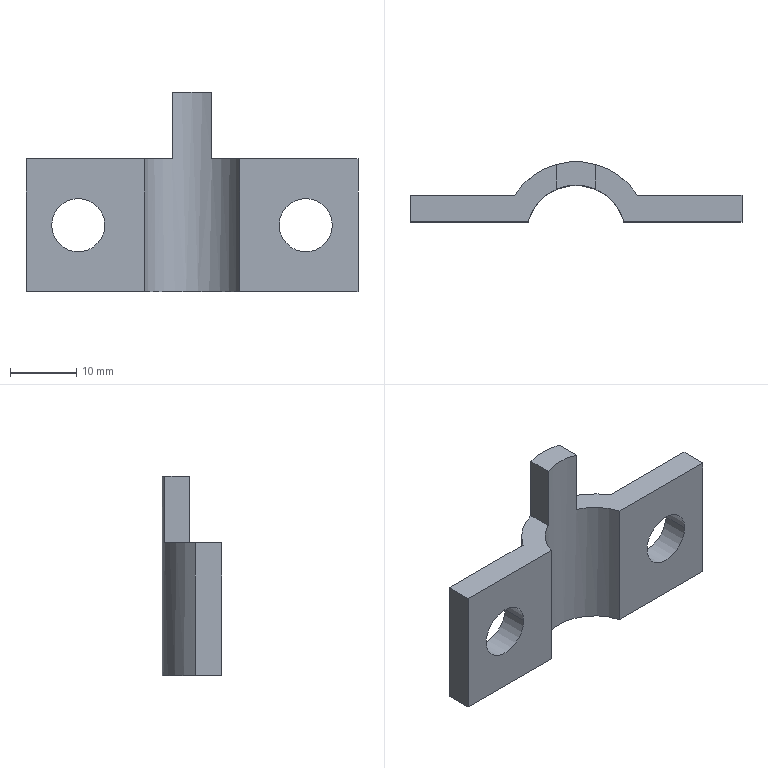Part | SolidWorks | features ICE 2, Extrusion 1 | 1 solid | 18 faces | box 50 x 9.031 x 30 mm | volume 3952 mm3 | plane 12 | cylinder 6 | commonest cylinder face diameters 8 x4 15 x1 22.063 x1
STEP:
#1=CARTESIAN_POINT('',(21.128,4.,10.));
#2=VERTEX_POINT('',#1);
#3=CARTESIAN_POINT('',(13.128,4.,10.));
#4=VERTEX_POINT('',#3);
#5=CARTESIAN_POINT('',(17.128,4.,10.));
#6=DIRECTION('',(0.,1.,0.));
#7=DIRECTION('',(-1.,0.,0.));
#8=AXIS2_PLACEMENT_3D('',#5,#6,#7);
#9=CIRCLE('',#8,4.);
#10=EDGE_CURVE('',#2,#4,#9,.T.);
#11=ORIENTED_EDGE('',*,*,#10,.F.);
#12=CARTESIAN_POINT('',(21.128,8.,10.));
#13=VERTEX_POINT('',#12);
#14=CARTESIAN_POINT('',(21.128,4.,10.));
#15=DIRECTION('',(0.,1.,0.));
#16=VECTOR('',#15,1000.);
#17=LINE('',#14,#16);
#18=EDGE_CURVE('',#2,#13,#17,.T.);
#19=ORIENTED_EDGE('',*,*,#18,.T.);
#20=CARTESIAN_POINT('',(13.128,8.,10.));
#21=VERTEX_POINT('',#20);
#22=CARTESIAN_POINT('',(17.128,8.,10.));
#23=DIRECTION('',(0.,1.,0.));
#24=DIRECTION('',(-1.,0.,0.));
#25=AXIS2_PLACEMENT_3D('',#22,#23,#24);
#26=CIRCLE('',#25,4.);
#27=EDGE_CURVE('',#13,#21,#26,.T.);
#28=ORIENTED_EDGE('',*,*,#27,.T.);
#29=CARTESIAN_POINT('',(13.128,4.,10.));
#30=DIRECTION('',(0.,1.,0.));
#31=VECTOR('',#30,1000.);
#32=LINE('',#29,#31);
#33=EDGE_CURVE('',#4,#21,#32,.T.);
#34=ORIENTED_EDGE('',*,*,#33,.F.);
#35=EDGE_LOOP('',(#11,#19,#28,#34));
#36=FACE_OUTER_BOUND('',#35,.T.);
#37=CARTESIAN_POINT('',(17.128,4.,10.));
#38=DIRECTION('',(0.,1.,0.));
#39=DIRECTION('',(-1.,0.,0.));
#40=AXIS2_PLACEMENT_3D('',#37,#38,#39);
#41=CYLINDRICAL_SURFACE('',#40,4.);
#42=ADVANCED_FACE('',(#36),#41,.F.);
#43=CARTESIAN_POINT('',(-13.128,4.,10.));
#44=VERTEX_POINT('',#43);
#45=CARTESIAN_POINT('',(-21.128,4.,10.));
#46=VERTEX_POINT('',#45);
#47=CARTESIAN_POINT('',(-17.128,4.,10.));
#48=DIRECTION('',(0.,1.,0.));
#49=DIRECTION('',(-1.,0.,0.));
#50=AXIS2_PLACEMENT_3D('',#47,#48,#49);
#51=CIRCLE('',#50,4.);
#52=EDGE_CURVE('',#44,#46,#51,.T.);
#53=ORIENTED_EDGE('',*,*,#52,.F.);
#54=CARTESIAN_POINT('',(-13.128,8.,10.));
#55=VERTEX_POINT('',#54);
#56=CARTESIAN_POINT('',(-13.128,4.,10.));
#57=DIRECTION('',(0.,1.,0.));
#58=VECTOR('',#57,1000.);
#59=LINE('',#56,#58);
#60=EDGE_CURVE('',#44,#55,#59,.T.);
#61=ORIENTED_EDGE('',*,*,#60,.T.);
#62=CARTESIAN_POINT('',(-21.128,8.,10.));
#63=VERTEX_POINT('',#62);
#64=CARTESIAN_POINT('',(-17.128,8.,10.));
#65=DIRECTION('',(0.,1.,0.));
#66=DIRECTION('',(-1.,0.,0.));
#67=AXIS2_PLACEMENT_3D('',#64,#65,#66);
#68=CIRCLE('',#67,4.);
#69=EDGE_CURVE('',#55,#63,#68,.T.);
#70=ORIENTED_EDGE('',*,*,#69,.T.);
#71=CARTESIAN_POINT('',(-21.128,4.,10.));
#72=DIRECTION('',(0.,1.,0.));
#73=VECTOR('',#72,1000.);
#74=LINE('',#71,#73);
#75=EDGE_CURVE('',#46,#63,#74,.T.);
#76=ORIENTED_EDGE('',*,*,#75,.F.);
#77=EDGE_LOOP('',(#53,#61,#70,#76));
#78=FACE_OUTER_BOUND('',#77,.T.);
#79=CARTESIAN_POINT('',(-17.128,4.,10.));
#80=DIRECTION('',(0.,1.,0.));
#81=DIRECTION('',(-1.,0.,0.));
#82=AXIS2_PLACEMENT_3D('',#79,#80,#81);
#83=CYLINDRICAL_SURFACE('',#82,4.);
#84=ADVANCED_FACE('',(#78),#83,.F.);
#85=CARTESIAN_POINT('',(7.228,4.,20.));
#86=VERTEX_POINT('',#85);
#87=CARTESIAN_POINT('',(7.228,4.,0.));
#88=VERTEX_POINT('',#87);
#89=CARTESIAN_POINT('',(7.228,4.,30.));
#90=DIRECTION('',(0.,0.,-1.));
#91=VECTOR('',#90,1000.);
#92=LINE('',#89,#91);
#93=EDGE_CURVE('',#86,#88,#92,.T.);
#94=ORIENTED_EDGE('',*,*,#93,.F.);
#95=CARTESIAN_POINT('',(3.,8.874,20.));
#96=VERTEX_POINT('',#95);
#97=CARTESIAN_POINT('',(0.,2.,20.));
#98=DIRECTION('',(0.,0.,1.));
#99=DIRECTION('',(-1.,0.,0.));
#100=AXIS2_PLACEMENT_3D('',#97,#98,#99);
#101=CIRCLE('',#100,7.5);
#102=EDGE_CURVE('',#86,#96,#101,.T.);
#103=ORIENTED_EDGE('',*,*,#102,.T.);
#104=CARTESIAN_POINT('',(3.,8.874,30.));
#105=VERTEX_POINT('',#104);
#106=CARTESIAN_POINT('',(3.,8.874,30.));
#107=DIRECTION('',(0.,0.,1.));
#108=VECTOR('',#107,1000.);
#109=LINE('',#106,#108);
#110=EDGE_CURVE('',#96,#105,#109,.T.);
#111=ORIENTED_EDGE('',*,*,#110,.T.);
#112=CARTESIAN_POINT('',(-3.,8.874,30.));
#113=VERTEX_POINT('',#112);
#114=CARTESIAN_POINT('',(0.,2.,30.));
#115=DIRECTION('',(0.,0.,-1.));
#116=DIRECTION('',(1.,0.,0.));
#117=AXIS2_PLACEMENT_3D('',#114,#115,#116);
#118=CIRCLE('',#117,7.5);
#119=EDGE_CURVE('',#113,#105,#118,.T.);
#120=ORIENTED_EDGE('',*,*,#119,.F.);
#121=CARTESIAN_POINT('',(-3.,8.874,20.));
#122=VERTEX_POINT('',#121);
#123=CARTESIAN_POINT('',(-3.,8.874,30.));
#124=DIRECTION('',(0.,0.,-1.));
#125=VECTOR('',#124,1000.);
#126=LINE('',#123,#125);
#127=EDGE_CURVE('',#113,#122,#126,.T.);
#128=ORIENTED_EDGE('',*,*,#127,.T.);
#129=CARTESIAN_POINT('',(-7.228,4.,20.));
#130=VERTEX_POINT('',#129);
#131=CARTESIAN_POINT('',(0.,2.,20.));
#132=DIRECTION('',(0.,0.,1.));
#133=DIRECTION('',(-1.,0.,0.));
#134=AXIS2_PLACEMENT_3D('',#131,#132,#133);
#135=CIRCLE('',#134,7.5);
#136=EDGE_CURVE('',#122,#130,#135,.T.);
#137=ORIENTED_EDGE('',*,*,#136,.T.);
#138=CARTESIAN_POINT('',(-7.228,4.,0.));
#139=VERTEX_POINT('',#138);
#140=CARTESIAN_POINT('',(-7.228,4.,30.));
#141=DIRECTION('',(0.,0.,-1.));
#142=VECTOR('',#141,1000.);
#143=LINE('',#140,#142);
#144=EDGE_CURVE('',#130,#139,#143,.T.);
#145=ORIENTED_EDGE('',*,*,#144,.T.);
#146=CARTESIAN_POINT('',(0.,2.,0.));
#147=DIRECTION('',(0.,0.,-1.));
#148=DIRECTION('',(1.,0.,0.));
#149=AXIS2_PLACEMENT_3D('',#146,#147,#148);
#150=CIRCLE('',#149,7.5);
#151=EDGE_CURVE('',#139,#88,#150,.T.);
#152=ORIENTED_EDGE('',*,*,#151,.T.);
#153=EDGE_LOOP('',(#94,#103,#111,#120,#128,#137,#145,#152));
#154=FACE_OUTER_BOUND('',#153,.T.);
#155=CARTESIAN_POINT('',(0.,2.,30.));
#156=DIRECTION('',(0.,0.,-1.));
#157=DIRECTION('',(-1.,0.,0.));
#158=AXIS2_PLACEMENT_3D('',#155,#156,#157);
#159=CYLINDRICAL_SURFACE('',#158,7.5);
#160=ADVANCED_FACE('',(#154),#159,.F.);
#161=CARTESIAN_POINT('',(17.128,4.,10.));
#162=DIRECTION('',(0.,1.,0.));
#163=DIRECTION('',(-1.,0.,0.));
#164=AXIS2_PLACEMENT_3D('',#161,#162,#163);
#165=CIRCLE('',#164,4.);
#166=EDGE_CURVE('',#4,#2,#165,.T.);
#167=ORIENTED_EDGE('',*,*,#166,.T.);
#168=ORIENTED_EDGE('',*,*,#10,.T.);
#169=EDGE_LOOP('',(#167,#168));
#170=FACE_BOUND('',#169,.T.);
#171=CARTESIAN_POINT('',(25.,4.,20.));
#172=VERTEX_POINT('',#171);
#173=CARTESIAN_POINT('',(25.,4.,0.));
#174=VERTEX_POINT('',#173);
#175=CARTESIAN_POINT('',(25.,4.,30.));
#176=DIRECTION('',(0.,0.,-1.));
#177=VECTOR('',#176,1000.);
#178=LINE('',#175,#177);
#179=EDGE_CURVE('',#172,#174,#178,.T.);
#180=ORIENTED_EDGE('',*,*,#179,.F.);
#181=CARTESIAN_POINT('',(3.,4.,20.));
#182=DIRECTION('',(1.,0.,0.));
#183=VECTOR('',#182,1000.);
#184=LINE('',#181,#183);
#185=EDGE_CURVE('',#86,#172,#184,.T.);
#186=ORIENTED_EDGE('',*,*,#185,.F.);
#187=ORIENTED_EDGE('',*,*,#93,.T.);
#188=CARTESIAN_POINT('',(7.228,4.,0.));
#189=DIRECTION('',(1.,0.,0.));
#190=VECTOR('',#189,1000.);
#191=LINE('',#188,#190);
#192=EDGE_CURVE('',#88,#174,#191,.T.);
#193=ORIENTED_EDGE('',*,*,#192,.T.);
#194=EDGE_LOOP('',(#180,#186,#187,#193));
#195=FACE_OUTER_BOUND('',#194,.T.);
#196=CARTESIAN_POINT('',(7.228,4.,30.));
#197=DIRECTION('',(0.,1.,0.));
#198=DIRECTION('',(0.,0.,1.));
#199=AXIS2_PLACEMENT_3D('',#196,#197,#198);
#200=PLANE('',#199);
#201=ADVANCED_FACE('',(#170,#195),#200,.F.);
#202=CARTESIAN_POINT('',(25.,8.,20.));
#203=VERTEX_POINT('',#202);
#204=CARTESIAN_POINT('',(25.,8.,0.));
#205=VERTEX_POINT('',#204);
#206=CARTESIAN_POINT('',(25.,8.,30.));
#207=DIRECTION('',(0.,0.,-1.));
#208=VECTOR('',#207,1000.);
#209=LINE('',#206,#208);
#210=EDGE_CURVE('',#203,#205,#209,.T.);
#211=ORIENTED_EDGE('',*,*,#210,.F.);
#212=CARTESIAN_POINT('',(25.,13.031,20.));
#213=DIRECTION('',(0.,-1.,0.));
#214=VECTOR('',#213,1000.);
#215=LINE('',#212,#214);
#216=EDGE_CURVE('',#203,#172,#215,.T.);
#217=ORIENTED_EDGE('',*,*,#216,.T.);
#218=ORIENTED_EDGE('',*,*,#179,.T.);
#219=CARTESIAN_POINT('',(25.,8.,0.));
#220=DIRECTION('',(0.,1.,0.));
#221=VECTOR('',#220,1000.);
#222=LINE('',#219,#221);
#223=EDGE_CURVE('',#174,#205,#222,.T.);
#224=ORIENTED_EDGE('',*,*,#223,.T.);
#225=EDGE_LOOP('',(#211,#217,#218,#224));
#226=FACE_OUTER_BOUND('',#225,.T.);
#227=CARTESIAN_POINT('',(25.,8.,30.));
#228=DIRECTION('',(-1.,0.,0.));
#229=DIRECTION('',(0.,0.,1.));
#230=AXIS2_PLACEMENT_3D('',#227,#228,#229);
#231=PLANE('',#230);
#232=ADVANCED_FACE('',(#226),#231,.F.);
#233=CARTESIAN_POINT('',(17.128,8.,10.));
#234=DIRECTION('',(0.,1.,0.));
#235=DIRECTION('',(-1.,0.,0.));
#236=AXIS2_PLACEMENT_3D('',#233,#234,#235);
#237=CIRCLE('',#236,4.);
#238=EDGE_CURVE('',#21,#13,#237,.T.);
#239=ORIENTED_EDGE('',*,*,#238,.F.);
#240=ORIENTED_EDGE('',*,*,#27,.F.);
#241=EDGE_LOOP('',(#239,#240));
#242=FACE_BOUND('',#241,.T.);
#243=CARTESIAN_POINT('',(9.257,8.,20.));
#244=VERTEX_POINT('',#243);
#245=CARTESIAN_POINT('',(9.257,8.,0.));
#246=VERTEX_POINT('',#245);
#247=CARTESIAN_POINT('',(9.257,8.,30.));
#248=DIRECTION('',(0.,0.,-1.));
#249=VECTOR('',#248,1000.);
#250=LINE('',#247,#249);
#251=EDGE_CURVE('',#244,#246,#250,.T.);
#252=ORIENTED_EDGE('',*,*,#251,.F.);
#253=CARTESIAN_POINT('',(25.,8.,20.));
#254=DIRECTION('',(1.,0.,0.));
#255=VECTOR('',#254,1000.);
#256=LINE('',#253,#255);
#257=EDGE_CURVE('',#244,#203,#256,.T.);
#258=ORIENTED_EDGE('',*,*,#257,.T.);
#259=ORIENTED_EDGE('',*,*,#210,.T.);
#260=CARTESIAN_POINT('',(25.,8.,0.));
#261=DIRECTION('',(-1.,0.,0.));
#262=VECTOR('',#261,1000.);
#263=LINE('',#260,#262);
#264=EDGE_CURVE('',#205,#246,#263,.T.);
#265=ORIENTED_EDGE('',*,*,#264,.T.);
#266=EDGE_LOOP('',(#252,#258,#259,#265));
#267=FACE_OUTER_BOUND('',#266,.T.);
#268=CARTESIAN_POINT('',(25.,8.,30.));
#269=DIRECTION('',(0.,-1.,0.));
#270=DIRECTION('',(1.,0.,0.));
#271=AXIS2_PLACEMENT_3D('',#268,#269,#270);
#272=PLANE('',#271);
#273=ADVANCED_FACE('',(#242,#267),#272,.F.);
#274=CARTESIAN_POINT('',(3.,12.616,30.));
#275=VERTEX_POINT('',#274);
#276=CARTESIAN_POINT('',(3.,12.616,20.));
#277=VERTEX_POINT('',#276);
#278=CARTESIAN_POINT('',(3.,12.616,30.));
#279=DIRECTION('',(0.,0.,-1.));
#280=VECTOR('',#279,1000.);
#281=LINE('',#278,#280);
#282=EDGE_CURVE('',#275,#277,#281,.T.);
#283=ORIENTED_EDGE('',*,*,#282,.T.);
#284=CARTESIAN_POINT('',(0.,2.,20.));
#285=DIRECTION('',(0.,0.,-1.));
#286=DIRECTION('',(-1.,0.,0.));
#287=AXIS2_PLACEMENT_3D('',#284,#285,#286);
#288=CIRCLE('',#287,11.031);
#289=EDGE_CURVE('',#277,#244,#288,.T.);
#290=ORIENTED_EDGE('',*,*,#289,.T.);
#291=ORIENTED_EDGE('',*,*,#251,.T.);
#292=CARTESIAN_POINT('',(-9.257,8.,0.));
#293=VERTEX_POINT('',#292);
#294=CARTESIAN_POINT('',(0.,2.,0.));
#295=DIRECTION('',(0.,0.,1.));
#296=DIRECTION('',(1.,0.,0.));
#297=AXIS2_PLACEMENT_3D('',#294,#295,#296);
#298=CIRCLE('',#297,11.031);
#299=EDGE_CURVE('',#246,#293,#298,.T.);
#300=ORIENTED_EDGE('',*,*,#299,.T.);
#301=CARTESIAN_POINT('',(-9.257,8.,20.));
#302=VERTEX_POINT('',#301);
#303=CARTESIAN_POINT('',(-9.257,8.,30.));
#304=DIRECTION('',(0.,0.,-1.));
#305=VECTOR('',#304,1000.);
#306=LINE('',#303,#305);
#307=EDGE_CURVE('',#302,#293,#306,.T.);
#308=ORIENTED_EDGE('',*,*,#307,.F.);
#309=CARTESIAN_POINT('',(-3.,12.616,20.));
#310=VERTEX_POINT('',#309);
#311=CARTESIAN_POINT('',(0.,2.,20.));
#312=DIRECTION('',(0.,0.,-1.));
#313=DIRECTION('',(-1.,0.,0.));
#314=AXIS2_PLACEMENT_3D('',#311,#312,#313);
#315=CIRCLE('',#314,11.031);
#316=EDGE_CURVE('',#302,#310,#315,.T.);
#317=ORIENTED_EDGE('',*,*,#316,.T.);
#318=CARTESIAN_POINT('',(-3.,12.616,30.));
#319=VERTEX_POINT('',#318);
#320=CARTESIAN_POINT('',(-3.,12.616,30.));
#321=DIRECTION('',(0.,0.,1.));
#322=VECTOR('',#321,1000.);
#323=LINE('',#320,#322);
#324=EDGE_CURVE('',#310,#319,#323,.T.);
#325=ORIENTED_EDGE('',*,*,#324,.T.);
#326=CARTESIAN_POINT('',(0.,2.,30.));
#327=DIRECTION('',(0.,0.,1.));
#328=DIRECTION('',(1.,0.,0.));
#329=AXIS2_PLACEMENT_3D('',#326,#327,#328);
#330=CIRCLE('',#329,11.031);
#331=EDGE_CURVE('',#275,#319,#330,.T.);
#332=ORIENTED_EDGE('',*,*,#331,.F.);
#333=EDGE_LOOP('',(#283,#290,#291,#300,#308,#317,#325,#332));
#334=FACE_OUTER_BOUND('',#333,.T.);
#335=CARTESIAN_POINT('',(0.,2.,30.));
#336=DIRECTION('',(0.,0.,-1.));
#337=DIRECTION('',(-1.,0.,0.));
#338=AXIS2_PLACEMENT_3D('',#335,#336,#337);
#339=CYLINDRICAL_SURFACE('',#338,11.031);
#340=ADVANCED_FACE('',(#334),#339,.T.);
#341=CARTESIAN_POINT('',(-17.128,8.,10.));
#342=DIRECTION('',(0.,1.,0.));
#343=DIRECTION('',(-1.,0.,0.));
#344=AXIS2_PLACEMENT_3D('',#341,#342,#343);
#345=CIRCLE('',#344,4.);
#346=EDGE_CURVE('',#63,#55,#345,.T.);
#347=ORIENTED_EDGE('',*,*,#346,.F.);
#348=ORIENTED_EDGE('',*,*,#69,.F.);
#349=EDGE_LOOP('',(#347,#348));
#350=FACE_BOUND('',#349,.T.);
#351=CARTESIAN_POINT('',(-25.,8.,20.));
#352=VERTEX_POINT('',#351);
#353=CARTESIAN_POINT('',(-25.,8.,0.));
#354=VERTEX_POINT('',#353);
#355=CARTESIAN_POINT('',(-25.,8.,30.));
#356=DIRECTION('',(0.,0.,-1.));
#357=VECTOR('',#356,1000.);
#358=LINE('',#355,#357);
#359=EDGE_CURVE('',#352,#354,#358,.T.);
#360=ORIENTED_EDGE('',*,*,#359,.F.);
#361=CARTESIAN_POINT('',(-25.,8.,20.));
#362=DIRECTION('',(1.,0.,0.));
#363=VECTOR('',#362,1000.);
#364=LINE('',#361,#363);
#365=EDGE_CURVE('',#352,#302,#364,.T.);
#366=ORIENTED_EDGE('',*,*,#365,.T.);
#367=ORIENTED_EDGE('',*,*,#307,.T.);
#368=CARTESIAN_POINT('',(-25.,8.,0.));
#369=DIRECTION('',(-1.,0.,0.));
#370=VECTOR('',#369,1000.);
#371=LINE('',#368,#370);
#372=EDGE_CURVE('',#293,#354,#371,.T.);
#373=ORIENTED_EDGE('',*,*,#372,.T.);
#374=EDGE_LOOP('',(#360,#366,#367,#373));
#375=FACE_OUTER_BOUND('',#374,.T.);
#376=CARTESIAN_POINT('',(-25.,8.,30.));
#377=DIRECTION('',(0.,-1.,0.));
#378=DIRECTION('',(0.,0.,-1.));
#379=AXIS2_PLACEMENT_3D('',#376,#377,#378);
#380=PLANE('',#379);
#381=ADVANCED_FACE('',(#350,#375),#380,.F.);
#382=CARTESIAN_POINT('',(-25.,4.,20.));
#383=VERTEX_POINT('',#382);
#384=CARTESIAN_POINT('',(-25.,4.,0.));
#385=VERTEX_POINT('',#384);
#386=CARTESIAN_POINT('',(-25.,4.,30.));
#387=DIRECTION('',(0.,0.,-1.));
#388=VECTOR('',#387,1000.);
#389=LINE('',#386,#388);
#390=EDGE_CURVE('',#383,#385,#389,.T.);
#391=ORIENTED_EDGE('',*,*,#390,.F.);
#392=CARTESIAN_POINT('',(-25.,13.031,20.));
#393=DIRECTION('',(0.,-1.,0.));
#394=VECTOR('',#393,1000.);
#395=LINE('',#392,#394);
#396=EDGE_CURVE('',#352,#383,#395,.T.);
#397=ORIENTED_EDGE('',*,*,#396,.F.);
#398=ORIENTED_EDGE('',*,*,#359,.T.);
#399=CARTESIAN_POINT('',(-25.,4.,0.));
#400=DIRECTION('',(0.,-1.,0.));
#401=VECTOR('',#400,1000.);
#402=LINE('',#399,#401);
#403=EDGE_CURVE('',#354,#385,#402,.T.);
#404=ORIENTED_EDGE('',*,*,#403,.T.);
#405=EDGE_LOOP('',(#391,#397,#398,#404));
#406=FACE_OUTER_BOUND('',#405,.T.);
#407=CARTESIAN_POINT('',(-25.,4.,30.));
#408=DIRECTION('',(1.,0.,0.));
#409=DIRECTION('',(0.,0.,-1.));
#410=AXIS2_PLACEMENT_3D('',#407,#408,#409);
#411=PLANE('',#410);
#412=ADVANCED_FACE('',(#406),#411,.F.);
#413=CARTESIAN_POINT('',(-17.128,4.,10.));
#414=DIRECTION('',(0.,1.,0.));
#415=DIRECTION('',(-1.,0.,0.));
#416=AXIS2_PLACEMENT_3D('',#413,#414,#415);
#417=CIRCLE('',#416,4.);
#418=EDGE_CURVE('',#46,#44,#417,.T.);
#419=ORIENTED_EDGE('',*,*,#418,.T.);
#420=ORIENTED_EDGE('',*,*,#52,.T.);
#421=EDGE_LOOP('',(#419,#420));
#422=FACE_BOUND('',#421,.T.);
#423=ORIENTED_EDGE('',*,*,#144,.F.);
#424=CARTESIAN_POINT('',(-25.,4.,20.));
#425=DIRECTION('',(1.,0.,0.));
#426=VECTOR('',#425,1000.);
#427=LINE('',#424,#426);
#428=EDGE_CURVE('',#383,#130,#427,.T.);
#429=ORIENTED_EDGE('',*,*,#428,.F.);
#430=ORIENTED_EDGE('',*,*,#390,.T.);
#431=CARTESIAN_POINT('',(-25.,4.,0.));
#432=DIRECTION('',(1.,0.,0.));
#433=VECTOR('',#432,1000.);
#434=LINE('',#431,#433);
#435=EDGE_CURVE('',#385,#139,#434,.T.);
#436=ORIENTED_EDGE('',*,*,#435,.T.);
#437=EDGE_LOOP('',(#423,#429,#430,#436));
#438=FACE_OUTER_BOUND('',#437,.T.);
#439=CARTESIAN_POINT('',(-25.,4.,30.));
#440=DIRECTION('',(0.,1.,0.));
#441=DIRECTION('',(-1.,0.,0.));
#442=AXIS2_PLACEMENT_3D('',#439,#440,#441);
#443=PLANE('',#442);
#444=ADVANCED_FACE('',(#422,#438),#443,.F.);
#445=CARTESIAN_POINT('',(3.,2.,30.));
#446=DIRECTION('',(0.,-1.,0.));
#447=VECTOR('',#446,1000.);
#448=LINE('',#445,#447);
#449=EDGE_CURVE('',#275,#105,#448,.T.);
#450=ORIENTED_EDGE('',*,*,#449,.F.);
#451=ORIENTED_EDGE('',*,*,#331,.T.);
#452=CARTESIAN_POINT('',(-3.,2.,30.));
#453=DIRECTION('',(0.,1.,0.));
#454=VECTOR('',#453,1000.);
#455=LINE('',#452,#454);
#456=EDGE_CURVE('',#113,#319,#455,.T.);
#457=ORIENTED_EDGE('',*,*,#456,.F.);
#458=ORIENTED_EDGE('',*,*,#119,.T.);
#459=EDGE_LOOP('',(#450,#451,#457,#458));
#460=FACE_OUTER_BOUND('',#459,.T.);
#461=CARTESIAN_POINT('',(0.,2.,30.));
#462=DIRECTION('',(0.,0.,1.));
#463=DIRECTION('',(1.,0.,0.));
#464=AXIS2_PLACEMENT_3D('',#461,#462,#463);
#465=PLANE('',#464);
#466=ADVANCED_FACE('',(#460),#465,.T.);
#467=ORIENTED_EDGE('',*,*,#151,.F.);
#468=ORIENTED_EDGE('',*,*,#435,.F.);
#469=ORIENTED_EDGE('',*,*,#403,.F.);
#470=ORIENTED_EDGE('',*,*,#372,.F.);
#471=ORIENTED_EDGE('',*,*,#299,.F.);
#472=ORIENTED_EDGE('',*,*,#264,.F.);
#473=ORIENTED_EDGE('',*,*,#223,.F.);
#474=ORIENTED_EDGE('',*,*,#192,.F.);
#475=EDGE_LOOP('',(#467,#468,#469,#470,#471,#472,#473,#474));
#476=FACE_OUTER_BOUND('',#475,.T.);
#477=CARTESIAN_POINT('',(0.,2.,0.));
#478=DIRECTION('',(0.,0.,1.));
#479=DIRECTION('',(1.,0.,0.));
#480=AXIS2_PLACEMENT_3D('',#477,#478,#479);
#481=PLANE('',#480);
#482=ADVANCED_FACE('',(#476),#481,.F.);
#483=CARTESIAN_POINT('',(-3.,13.031,20.));
#484=DIRECTION('',(0.,-1.,0.));
#485=VECTOR('',#484,1000.);
#486=LINE('',#483,#485);
#487=EDGE_CURVE('',#310,#122,#486,.T.);
#488=ORIENTED_EDGE('',*,*,#487,.F.);
#489=ORIENTED_EDGE('',*,*,#316,.F.);
#490=ORIENTED_EDGE('',*,*,#365,.F.);
#491=ORIENTED_EDGE('',*,*,#396,.T.);
#492=ORIENTED_EDGE('',*,*,#428,.T.);
#493=ORIENTED_EDGE('',*,*,#136,.F.);
#494=EDGE_LOOP('',(#488,#489,#490,#491,#492,#493));
#495=FACE_OUTER_BOUND('',#494,.T.);
#496=CARTESIAN_POINT('',(-25.,13.031,20.));
#497=DIRECTION('',(0.,0.,-1.));
#498=DIRECTION('',(-1.,0.,0.));
#499=AXIS2_PLACEMENT_3D('',#496,#497,#498);
#500=PLANE('',#499);
#501=ADVANCED_FACE('',(#495),#500,.F.);
#502=ORIENTED_EDGE('',*,*,#456,.T.);
#503=ORIENTED_EDGE('',*,*,#324,.F.);
#504=ORIENTED_EDGE('',*,*,#487,.T.);
#505=ORIENTED_EDGE('',*,*,#127,.F.);
#506=EDGE_LOOP('',(#502,#503,#504,#505));
#507=FACE_OUTER_BOUND('',#506,.T.);
#508=CARTESIAN_POINT('',(-3.,13.031,20.));
#509=DIRECTION('',(1.,0.,0.));
#510=DIRECTION('',(0.,1.,0.));
#511=AXIS2_PLACEMENT_3D('',#508,#509,#510);
#512=PLANE('',#511);
#513=ADVANCED_FACE('',(#507),#512,.F.);
#514=ORIENTED_EDGE('',*,*,#185,.T.);
#515=ORIENTED_EDGE('',*,*,#216,.F.);
#516=ORIENTED_EDGE('',*,*,#257,.F.);
#517=ORIENTED_EDGE('',*,*,#289,.F.);
#518=CARTESIAN_POINT('',(3.,13.031,20.));
#519=DIRECTION('',(0.,-1.,0.));
#520=VECTOR('',#519,1000.);
#521=LINE('',#518,#520);
#522=EDGE_CURVE('',#277,#96,#521,.T.);
#523=ORIENTED_EDGE('',*,*,#522,.T.);
#524=ORIENTED_EDGE('',*,*,#102,.F.);
#525=EDGE_LOOP('',(#514,#515,#516,#517,#523,#524));
#526=FACE_OUTER_BOUND('',#525,.T.);
#527=CARTESIAN_POINT('',(3.,13.031,20.));
#528=DIRECTION('',(0.,0.,-1.));
#529=DIRECTION('',(-1.,0.,0.));
#530=AXIS2_PLACEMENT_3D('',#527,#528,#529);
#531=PLANE('',#530);
#532=ADVANCED_FACE('',(#526),#531,.F.);
#533=ORIENTED_EDGE('',*,*,#522,.F.);
#534=ORIENTED_EDGE('',*,*,#282,.F.);
#535=ORIENTED_EDGE('',*,*,#449,.T.);
#536=ORIENTED_EDGE('',*,*,#110,.F.);
#537=EDGE_LOOP('',(#533,#534,#535,#536));
#538=FACE_OUTER_BOUND('',#537,.T.);
#539=CARTESIAN_POINT('',(3.,13.031,30.));
#540=DIRECTION('',(-1.,0.,0.));
#541=DIRECTION('',(0.,0.,1.));
#542=AXIS2_PLACEMENT_3D('',#539,#540,#541);
#543=PLANE('',#542);
#544=ADVANCED_FACE('',(#538),#543,.F.);
#545=ORIENTED_EDGE('',*,*,#60,.F.);
#546=ORIENTED_EDGE('',*,*,#418,.F.);
#547=ORIENTED_EDGE('',*,*,#75,.T.);
#548=ORIENTED_EDGE('',*,*,#346,.T.);
#549=EDGE_LOOP('',(#545,#546,#547,#548));
#550=FACE_OUTER_BOUND('',#549,.T.);
#551=CARTESIAN_POINT('',(-17.128,4.,10.));
#552=DIRECTION('',(0.,1.,0.));
#553=DIRECTION('',(-1.,0.,0.));
#554=AXIS2_PLACEMENT_3D('',#551,#552,#553);
#555=CYLINDRICAL_SURFACE('',#554,4.);
#556=ADVANCED_FACE('',(#550),#555,.F.);
#557=ORIENTED_EDGE('',*,*,#18,.F.);
#558=ORIENTED_EDGE('',*,*,#166,.F.);
#559=ORIENTED_EDGE('',*,*,#33,.T.);
#560=ORIENTED_EDGE('',*,*,#238,.T.);
#561=EDGE_LOOP('',(#557,#558,#559,#560));
#562=FACE_OUTER_BOUND('',#561,.T.);
#563=CARTESIAN_POINT('',(17.128,4.,10.));
#564=DIRECTION('',(0.,1.,0.));
#565=DIRECTION('',(-1.,0.,0.));
#566=AXIS2_PLACEMENT_3D('',#563,#564,#565);
#567=CYLINDRICAL_SURFACE('',#566,4.);
#568=ADVANCED_FACE('',(#562),#567,.F.);
#569=CLOSED_SHELL('',(#42,#84,#160,#201,#232,#273,#340,#381,#412,#444,#466,#482,#501,#513,#532,#544,#556,#568));
#570=MANIFOLD_SOLID_BREP('',#569);
#571=CARTESIAN_POINT('',(0.,0.,0.));
#572=DIRECTION('',(0.,0.,1.));
#573=DIRECTION('',(1.,0.,0.));
#574=AXIS2_PLACEMENT_3D('',#571,#572,#573);
#575=(LENGTH_UNIT()NAMED_UNIT(*)SI_UNIT(.MILLI.,.METRE.));
#576=UNCERTAINTY_MEASURE_WITH_UNIT(LENGTH_MEASURE(0.00001),#575,'','');
#577=(NAMED_UNIT(*)PLANE_ANGLE_UNIT()SI_UNIT($,.RADIAN.));
#578=(NAMED_UNIT(*)SI_UNIT($,.STERADIAN.)SOLID_ANGLE_UNIT());
#579=(GEOMETRIC_REPRESENTATION_CONTEXT(3)GLOBAL_UNCERTAINTY_ASSIGNED_CONTEXT((#576))GLOBAL_UNIT_ASSIGNED_CONTEXT((#575,#577,#578))REPRESENTATION_CONTEXT('',''));
#580=ADVANCED_BREP_SHAPE_REPRESENTATION('',(#570,#574),#579);